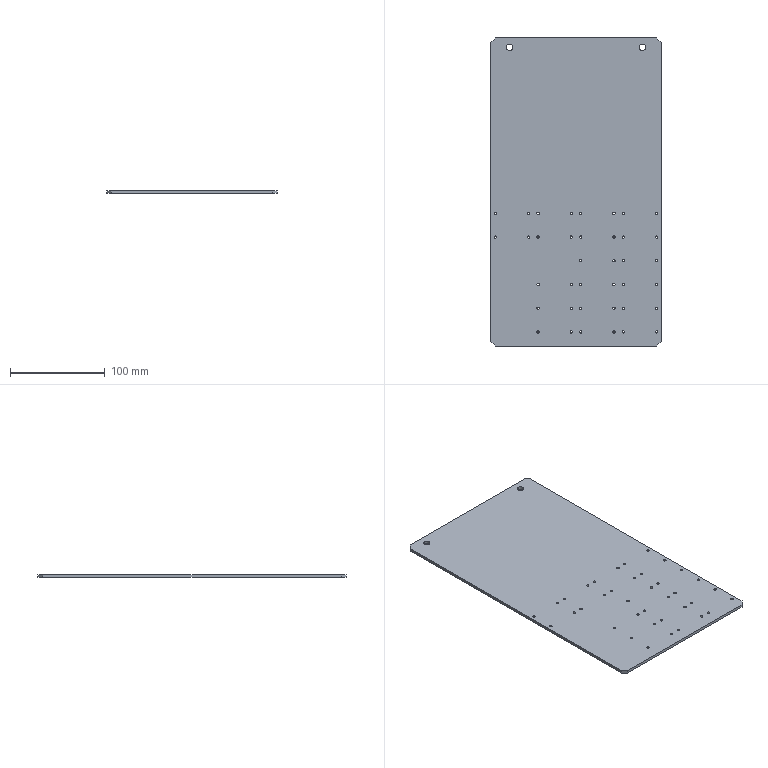Part | STEP file | J459-EBZ05-01-04-Part-1 | 1 solid | 90 faces | box 180 x 325 x 3 mm | volume 174573 mm3 | cylinder 80 | plane 10 | commonest cylinder face diameters 2.5 x76 6.8 x4